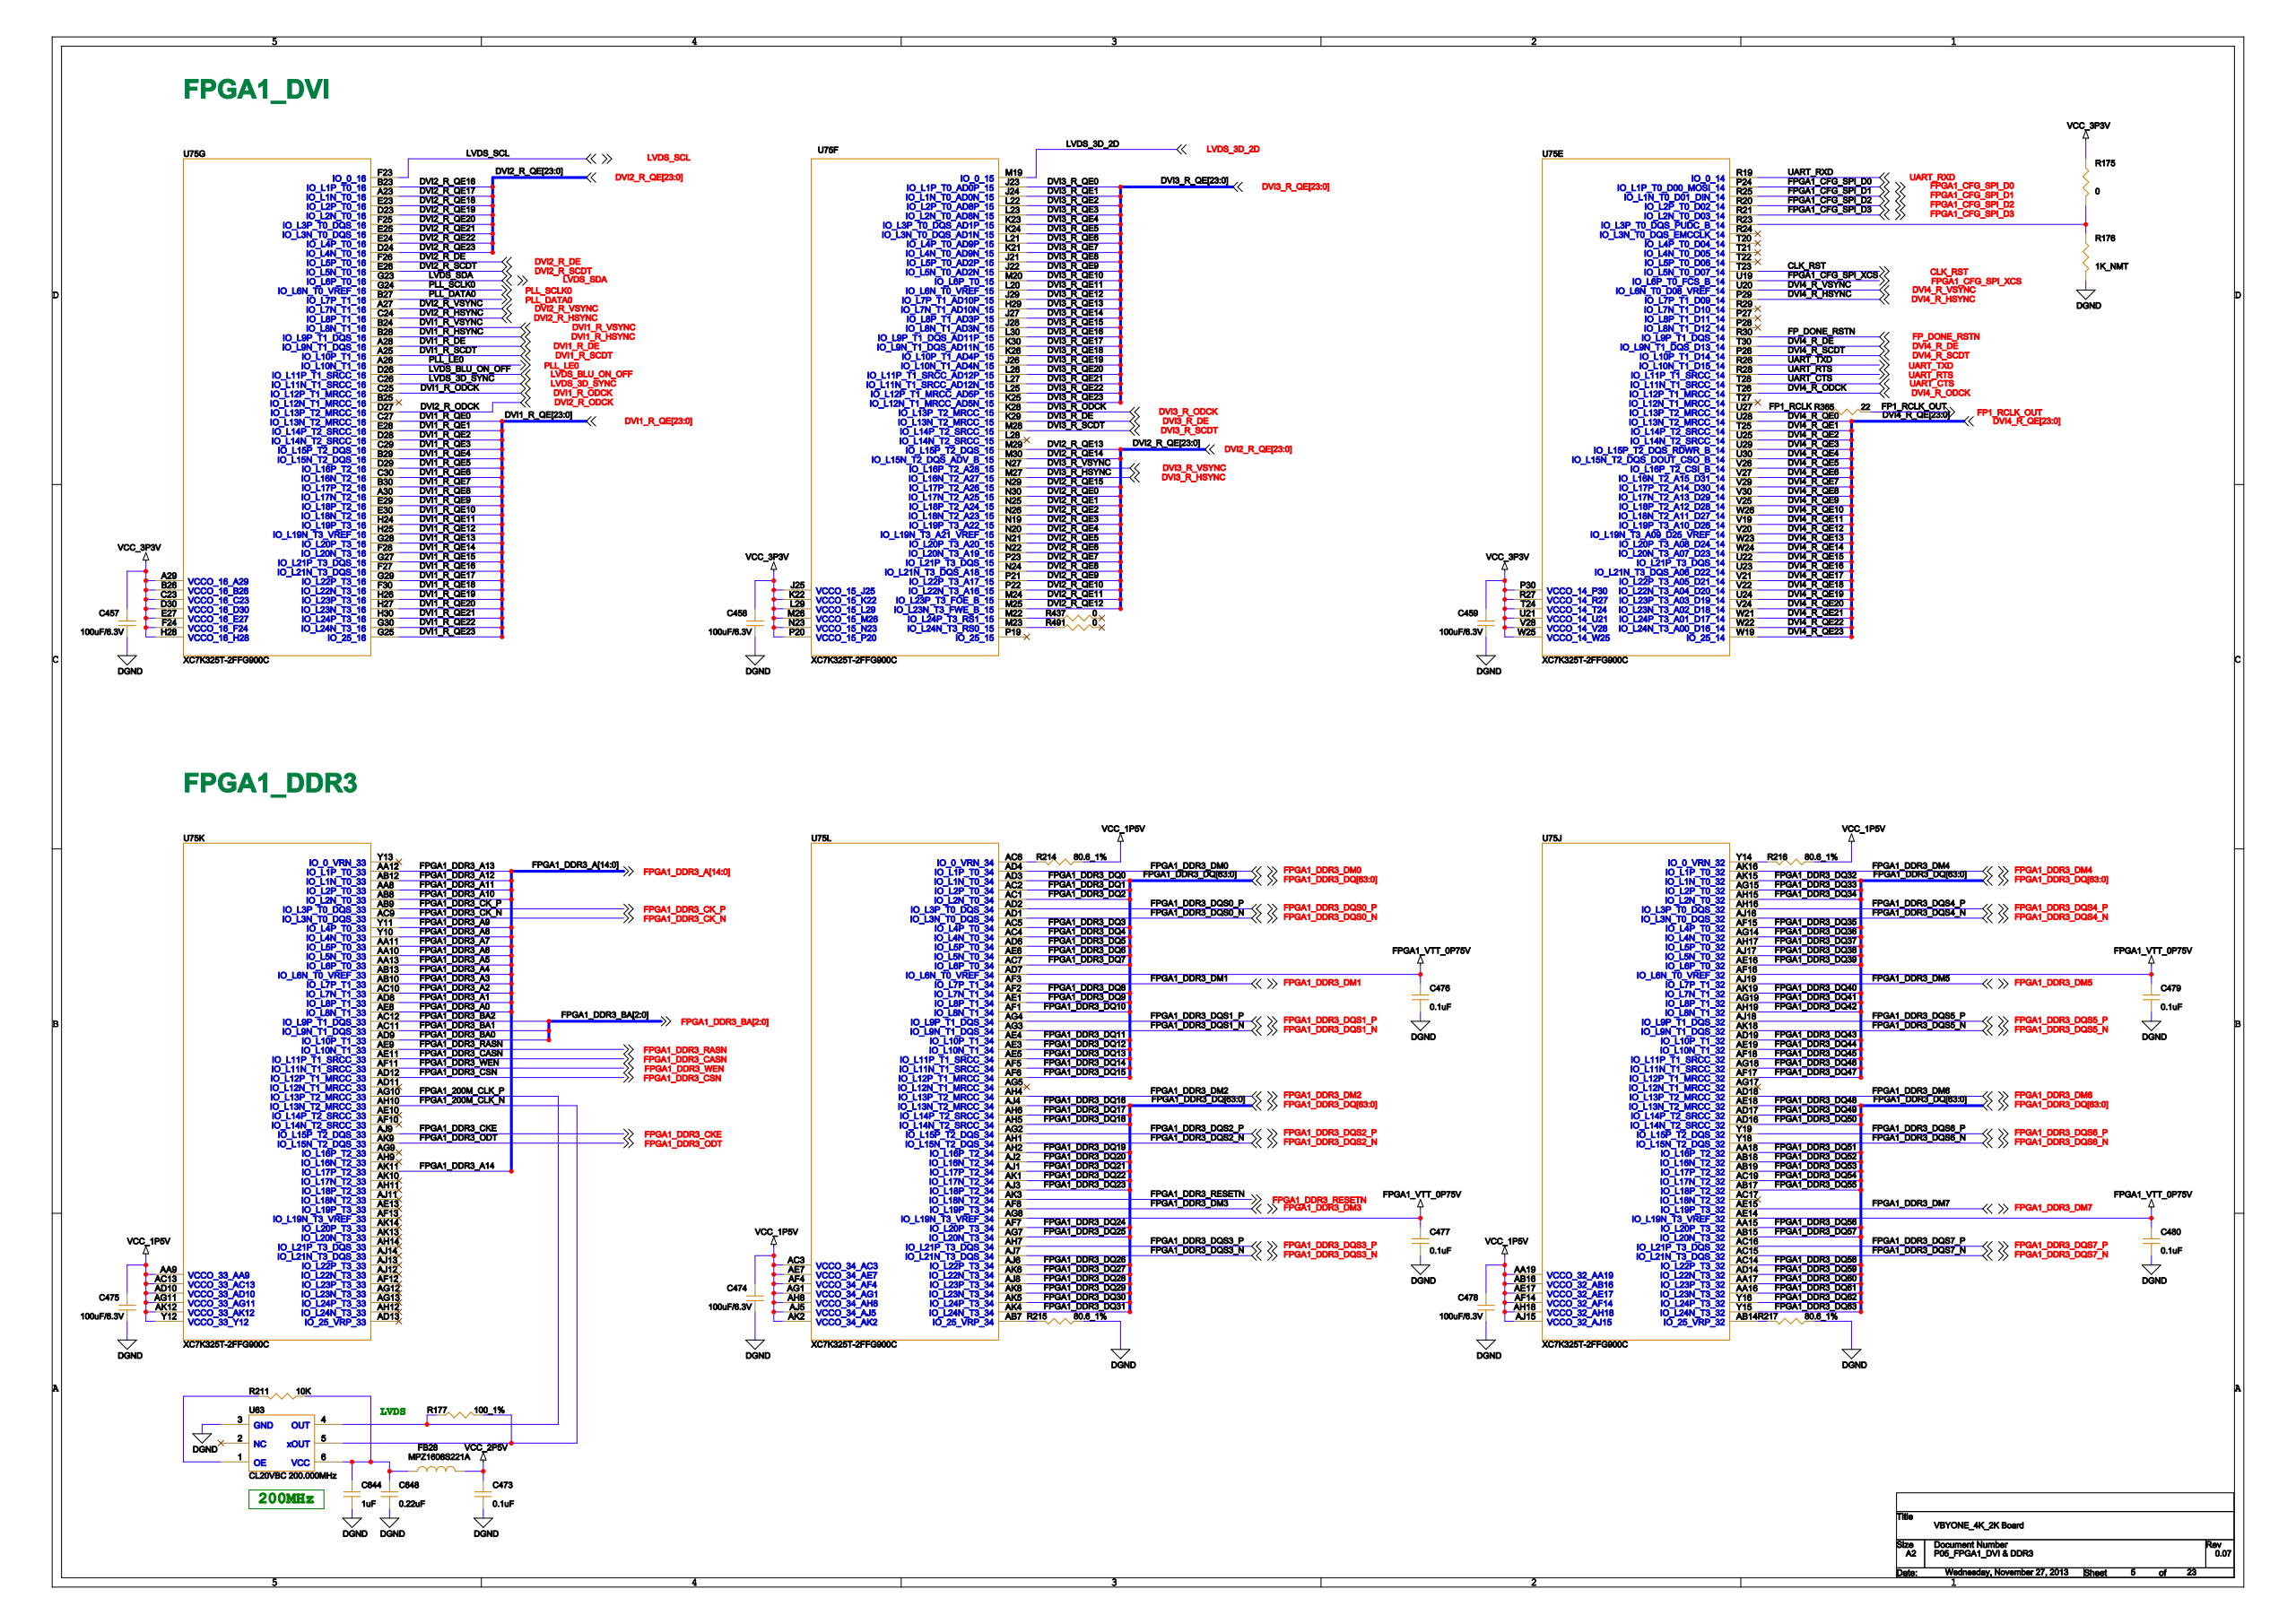Circuit board | Cadence Allegro | 1712 parts | 1495 nets | one sheet of the schematic
Parts on this sheet (reference | value | footprint):
C457 | 100uF/6.3V | CRC3225RZAS
C458 | 100uF/6.3V | CRC3225RZAS
C459 | 100uF/6.3V | CRC3225RZAS
C473 | 0.1uF | CRC1005RZAS
C474 | 100uF/6.3V | CRC3225RZAS
C475 | 100uF/6.3V | CRC3225RZAS
C476 | 0.1uF | CRC1005RZAS
C477 | 0.1uF | CRC1005RZAS
C478 | 100uF/6.3V | CRC3225RZAS
C479 | 0.1uF | CRC1005RZAS
C480 | 0.1uF | CRC1005RZAS
C644 | 1uF | CRC1608RZAS
C648 | 0.22uF | CRC1608RZAS
FB28 | MPZ1608S221A | LSC1608RZAS
R175 | 0 | CRC1608RZAS
R176 | 1K_NMT | CRC1608RZAS
R177 | 100_1% | CRC1005RZAS
R211 | 10K | CRC1005RZAS
R214 | 80.6_1% | CRC1608RZAS
R215 | 80.6_1% | CRC1608RZAS
R216 | 80.6_1% | CRC1608RZAS
R217 | 80.6_1% | CRC1608RZAS
R365 | 22 | CRC1005RZAS
R437 | 0 | CRC1608RZAS
R491 | 0 | CRC1608RZAS
U20 | LMK03033CISQ | QFN048RCBS
U21 | K4B4G1646B-HCK0 | BGA096RFDS
U22 | K4B4G1646B-HCK0 | BGA096RFDS
U23 | K4B4G1646B-HCK0 | BGA096RFDS
U24 | K4B4G1646B-HCK0 | BGA096RFDS
U63 | CL20VBC 200.000MHz | XTC006RLDS
U75 | XC7K325T-2FFG900C | BGA900RGAS
Nets of these parts (net: part-pin ...):
VCC_3P3V: C457-2 C458-2 C459-2 R175-1 U75-A29 U75-B26 U75-C23 U75-D30 U75-E27 U75-F24 U75-H28 U75-J25 U75-K22 U75-L29 U75-M26 U75-N23 U75-P20 U75-P30 U75-R27 U75-T24 U75-U21 U75-V28 U75-W25
DGND: C457-1 C458-1 C459-1 C473-2 C474-1 C475-1 C476-2 C477-2 C478-1 C479-2 C480-2 C644-2 C648-2 R176-2 R215-1 R217-1 U63-3 U20-1 U75-A2
VCC_1P5V: C474-2 C475-2 C478-2 R214-1 R216-1 U75-AA9 U75-AA19 U75-AB16 U75-AC3 U75-AC13 U75-AD10 U75-AE7 U75-AE17 U75-AF4 U75-AF14 U75-AG1 U75-AG11 U75-AH8 U75-AH18 U75-AJ5 U75-AJ15 U75-AK2 U75-AK12 U75-Y12
FPGA1_VTT_0P75V: C476-1 C477-1 C479-1 C480-1 U75-AD7 U75-AE14 U75-AF16 U75-AG8
VCC_2P5V: C473-1 FB28-2
N18157711: C644-1 C648-1 FB28-1 R211-1 U63-6
FP1_RCLK_OUT: R365-2
LVDS_SDA: U75-G23
LVDS_SCL: U75-F23
LVDS_3D_SYNC: U75-C26
LVDS_3D_2D: U75-M19
DVI1_R_ODCK: U75-C25
DVI3_R_DE: U75-K29
DVI3_R_VSYNC: U75-N27
DVI3_R_HSYNC: U75-M27
DVI4_R_ODCK: U75-T26
DVI4_R_DE: U75-T30
DVI4_R_VSYNC: U75-U20
DVI4_R_HSYNC: U75-P29
DVI1_R_DE: U75-A28
DVI1_R_VSYNC: U75-B24
DVI1_R_HSYNC: U75-B28
DVI2_R_ODCK: U75-D27
DVI2_R_DE: U75-F26
DVI2_R_VSYNC: U75-A27
DVI2_R_HSYNC: U75-C24
DVI3_R_ODCK: U75-K28
N16146863: R175-2 R176-1 U75-R23
N19425575: R437-1 U75-M22
N19425578: R491-1 U75-M23
FPGA1_200M_CLK_P: R177-1 U63-4 U75-AG10
FPGA1_200M_CLK_N: R177-2 U63-5 U75-AH10
FPGA1_CFG_SPI_D0: U75-P24
FPGA1_CFG_SPI_D1: U75-R25
FPGA1_CFG_SPI_D2: U75-R20
FPGA1_CFG_SPI_D3: U75-R21
FP_DONE_RSTN: U75-R30
FPGA1_DDR3_CKE: U75-AJ9
FPGA1_DDR3_RESETN: U75-AK3
CLK_RST: U75-T23
FPGA1_DDR3_ODT: U75-AK9
FPGA1_DDR3_CSN: U75-AD12
N18157807: R211-2 U63-1
FPGA1_DDR3_A0: U75-AE8
FPGA1_DDR3_A1: U75-AD8
FPGA1_DDR3_A2: U75-AC10
FPGA1_DDR3_A3: U75-AB10
FPGA1_DDR3_A4: U75-AB13
FPGA1_DDR3_A5: U75-AA13
FPGA1_DDR3_A6: U75-AA10
FPGA1_DDR3_A7: U75-AA11
FPGA1_DDR3_A8: U75-Y10
FPGA1_DDR3_A9: U75-Y11
FPGA1_DDR3_A10: U75-AB8
FPGA1_DDR3_A11: U75-AA8
FPGA1_DDR3_A12: U75-AB12
FPGA1_DDR3_A13: U75-AA12
FPGA1_DDR3_BA0: U75-AD9
FPGA1_DDR3_BA1: U75-AC11
FPGA1_DDR3_BA2: U75-AC12
FPGA1_DDR3_A14: U75-AK11
FPGA1_DDR3_RASN: U75-AE9
FPGA1_DDR3_CASN: U75-AE11
FPGA1_DDR3_WEN: U75-AF11
FPGA1_DDR3_CK_P: U75-AB9
FPGA1_DDR3_CK_N: U75-AC9
N17011473: R214-2 U75-AC6
N17011603: R215-2 U75-AB7
N17018638: R216-2 U75-Y14
N17018690: R217-2 U75-AB14
FPGA1_CFG_SPI_XCS: U75-U19
FP1_RCLK: R365-1 U75-U27
DVI2_R_SCDT: U75-E26
DVI2_R_QE0: U75-N30
DVI2_R_QE2: U75-N26
DVI2_R_QE1: U75-N25
DVI2_R_QE3: U75-N19
DVI2_R_QE4: U75-N20
DVI2_R_QE6: U75-N22
DVI2_R_QE5: U75-N21
DVI2_R_QE7: U75-P23
DVI2_R_QE8: U75-N24
DVI2_R_QE9: U75-P21
DVI2_R_QE10: U75-P22
DVI2_R_QE12: U75-M25
DVI2_R_QE11: U75-M24
DVI2_R_QE13: U75-M29
DVI2_R_QE14: U75-M30
DVI2_R_QE15: U75-N29
DVI2_R_QE16: U75-B23
DVI2_R_QE17: U75-A23
DVI2_R_QE19: U75-D23
DVI2_R_QE18: U75-E23
DVI2_R_QE20: U75-F25
DVI2_R_QE21: U75-E25
DVI2_R_QE23: U75-D24
DVI2_R_QE22: U75-E24
DVI3_R_SCDT: U75-M28
DVI3_R_QE0: U75-J23
DVI3_R_QE2: U75-L22
DVI3_R_QE1: U75-J24
DVI3_R_QE3: U75-L23
DVI3_R_QE4: U75-K23
DVI3_R_QE6: U75-L21
DVI3_R_QE5: U75-K24
DVI3_R_QE7: U75-K21
DVI3_R_QE8: U75-J21
DVI3_R_QE9: U75-J22
DVI3_R_QE10: U75-M20
DVI3_R_QE12: U75-J29
DVI3_R_QE11: U75-L20
DVI3_R_QE13: U75-H29
DVI3_R_QE14: U75-J27
DVI3_R_QE15: U75-J28
DVI3_R_QE16: U75-L30
DVI3_R_QE17: U75-K30
DVI3_R_QE19: U75-J26
DVI3_R_QE18: U75-K26
DVI3_R_QE20: U75-L26
DVI3_R_QE21: U75-L27
DVI3_R_QE23: U75-K25
DVI3_R_QE22: U75-L25
DVI4_R_SCDT: U75-P26
DVI4_R_QE0: U75-U28
DVI4_R_QE2: U75-U25
DVI4_R_QE1: U75-T25
DVI4_R_QE3: U75-U29
DVI4_R_QE4: U75-U30
DVI4_R_QE6: U75-V27
DVI4_R_QE5: U75-V26
DVI4_R_QE7: U75-V29
DVI4_R_QE8: U75-V30
DVI4_R_QE9: U75-V25
DVI4_R_QE10: U75-W26
DVI4_R_QE12: U75-V20
DVI4_R_QE11: U75-V19
DVI4_R_QE13: U75-W23
DVI4_R_QE14: U75-W24
DVI4_R_QE15: U75-U22
DVI4_R_QE16: U75-U23
DVI4_R_QE17: U75-V21
DVI4_R_QE19: U75-U24
DVI4_R_QE18: U75-V22
DVI4_R_QE20: U75-V24
DVI4_R_QE21: U75-W21
DVI4_R_QE23: U75-W19
DVI4_R_QE22: U75-W22
DVI1_R_SCDT: U75-A25
DVI1_R_QE0: U75-C27
DVI1_R_QE2: U75-D28
DVI1_R_QE1: U75-E28
DVI1_R_QE3: U75-C29
DVI1_R_QE4: U75-B29
DVI1_R_QE6: U75-C30
DVI1_R_QE5: U75-D29
DVI1_R_QE7: U75-B30
DVI1_R_QE8: U75-A30
DVI1_R_QE9: U75-E29
DVI1_R_QE10: U75-E30
DVI1_R_QE12: U75-H25
DVI1_R_QE11: U75-H24
DVI1_R_QE13: U75-G28
DVI1_R_QE14: U75-F28
DVI1_R_QE15: U75-G27
DVI1_R_QE16: U75-F27
DVI1_R_QE17: U75-G29
DVI1_R_QE19: U75-H26
DVI1_R_QE18: U75-F30
DVI1_R_QE20: U75-H27
DVI1_R_QE21: U75-H30
DVI1_R_QE23: U75-G25
DVI1_R_QE22: U75-G30
LVDS_BLU_ON_OFF: U75-D26
FPGA1_DDR3_DQ22: U75-AK1
FPGA1_DDR3_DQ21: U75-AJ1
FPGA1_DDR3_DQS2_N: U75-AH1
FPGA1_DDR3_DQ10: U75-AF1
FPGA1_DDR3_DQ9: U75-AE1
FPGA1_DDR3_DQS0_N: U75-AD1
FPGA1_DDR3_DQ2: U75-AC1
FPGA1_DDR3_DQ20: U75-AJ2
FPGA1_DDR3_DQ19: U75-AH2
FPGA1_DDR3_DQS2_P: U75-AG2
FPGA1_DDR3_DQ8: U75-AF2
FPGA1_DDR3_DQS0_P: U75-AD2
FPGA1_DDR3_DQ1: U75-AC2
FPGA1_DDR3_DQ23: U75-AJ3
FPGA1_DDR3_DQS1_N: U75-AG3
FPGA1_DDR3_DM1: U75-AF3
FPGA1_DDR3_DQ12: U75-AE3
FPGA1_DDR3_DQ0: U75-AD3
FPGA1_DDR3_DQ31: U75-AK4
FPGA1_DDR3_DQ16: U75-AJ4
FPGA1_DDR3_DM2: U75-AH4
FPGA1_DDR3_DQS1_P: U75-AG4
FPGA1_DDR3_DQ11: U75-AE4
FPGA1_DDR3_DM0: U75-AD4
FPGA1_DDR3_DQ4: U75-AC4
FPGA1_DDR3_DQ30: U75-AK5
FPGA1_DDR3_DQ18: U75-AH5
FPGA1_DDR3_DQ14: U75-AF5
FPGA1_DDR3_DQ13: U21-A2 U75-AE5
FPGA1_DDR3_DQ3: U75-AC5
FPGA1_DDR3_DQ27: U75-AK6
FPGA1_DDR3_DQ26: U75-AJ6
FPGA1_DDR3_DQ17: U75-AH6
FPGA1_DDR3_DQ15: U75-AF6
FPGA1_DDR3_DQ6: U75-AE6
FPGA1_DDR3_DQ5: U75-AD6
FPGA1_DDR3_DQS3_N: U75-AJ7
FPGA1_DDR3_DQS3_P: U75-AH7
FPGA1_DDR3_DQ25: U75-AG7
FPGA1_DDR3_DQ24: U75-AF7
FPGA1_DDR3_DQ7: U75-AC7
FPGA1_DDR3_DQ29: U22-A2 U75-AK8
FPGA1_DDR3_DQ28: U75-AJ8
FPGA1_DDR3_DM3: U75-AF8
FPGA1_DDR3_DQ36: U75-AG14
FPGA1_DDR3_DQ59: U75-AD14
FPGA1_DDR3_DQ58: U75-AC14
FPGA1_DDR3_DQ32: U75-AK15
FPGA1_DDR3_DQ34: U75-AH15
FPGA1_DDR3_DQ33: U75-AG15
FPGA1_DDR3_DQ35: U75-AF15
FPGA1_DDR3_DM7: U75-AE15
FPGA1_DDR3_DQS7_N: U75-AC15
FPGA1_DDR3_DQ57: U75-AB15
FPGA1_DDR3_DQ56: U75-AA15
FPGA1_DDR3_DQ63: U75-Y15
FPGA1_DDR3_DM4: U75-AK16
FPGA1_DDR3_DQS4_N: U75-AJ16
FPGA1_DDR3_DQS4_P: U75-AH16
FPGA1_DDR3_DQ39: U75-AE16
FPGA1_DDR3_DQ50: U75-AD16
FPGA1_DDR3_DQS7_P: U75-AC16
FPGA1_DDR3_DQ61: U24-A2 U75-AA16
FPGA1_DDR3_DQ62: U75-Y16
FPGA1_DDR3_DQ38: U75-AJ17
FPGA1_DDR3_DQ37: U75-AH17
FPGA1_DDR3_DQ47: U75-AF17
FPGA1_DDR3_DQ49: U75-AD17
FPGA1_DDR3_DQ55: U75-AB17
FPGA1_DDR3_DQ60: U75-AA17
FPGA1_DDR3_DQS5_N: U75-AK18
FPGA1_DDR3_DQS5_P: U75-AJ18
FPGA1_DDR3_DQ46: U75-AG18
FPGA1_DDR3_DQ45: U23-A2 U75-AF18
FPGA1_DDR3_DQ48: U75-AE18
FPGA1_DDR3_DM6: U75-AD18
FPGA1_DDR3_DQ52: U75-AB18
FPGA1_DDR3_DQ51: U75-AA18
FPGA1_DDR3_DQS6_N: U75-Y18
FPGA1_DDR3_DQ40: U75-AK19
FPGA1_DDR3_DM5: U75-AJ19
FPGA1_DDR3_DQ42: U75-AH19
FPGA1_DDR3_DQ41: U75-AG19
FPGA1_DDR3_DQ44: U75-AE19
FPGA1_DDR3_DQ43: U75-AD19
FPGA1_DDR3_DQ54: U75-AC19
FPGA1_DDR3_DQ53: U75-AB19
FPGA1_DDR3_DQS6_P: U75-Y19
UART_RXD: U75-R19
PLL_SCLK0: U20-4 U75-G24
UART_TXD: U75-R26
PLL_LE0: U20-6 U75-A26
PLL_DATA0: U20-5 U75-B27
UART_CTS: U75-T28
UART_RTS: U75-R28